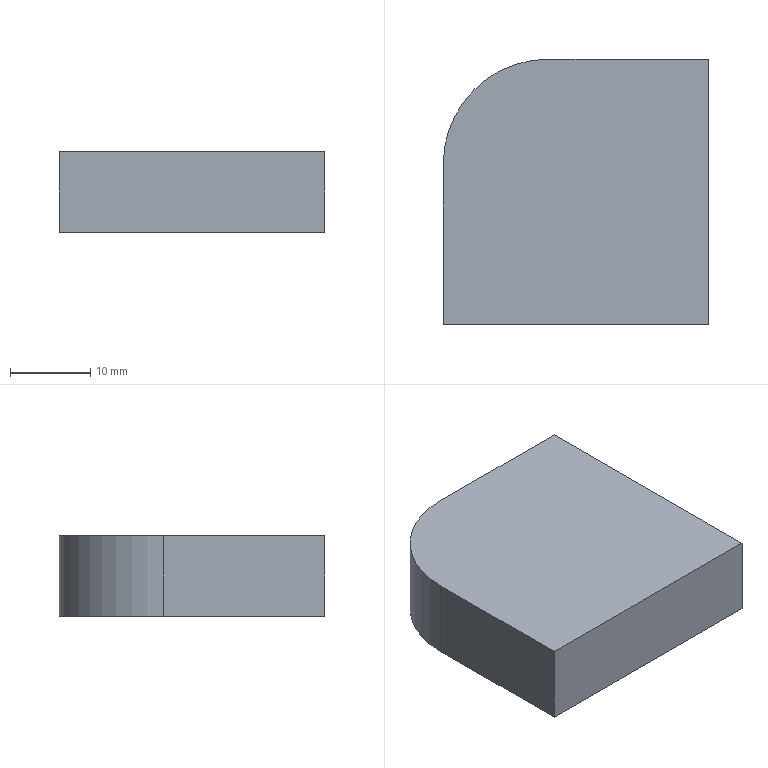Part | SolidWorks | features Extrusion 1, Fillet 1, ICE 1 | 1 solid | 7 faces | box 33 x 33 x 10 mm | volume 10527 mm3 | plane 6 | cylinder 1 | commonest cylinder face diameters 26 x1
STEP:
#1=CARTESIAN_POINT('',(7.,0.,10.));
#2=VERTEX_POINT('',#1);
#3=CARTESIAN_POINT('',(40.,0.,10.));
#4=VERTEX_POINT('',#3);
#5=CARTESIAN_POINT('',(40.,0.,10.));
#6=DIRECTION('',(1.,0.,0.));
#7=VECTOR('',#6,1000.);
#8=LINE('',#5,#7);
#9=EDGE_CURVE('',#2,#4,#8,.T.);
#10=ORIENTED_EDGE('',*,*,#9,.F.);
#11=CARTESIAN_POINT('',(7.,0.,0.));
#12=VERTEX_POINT('',#11);
#13=CARTESIAN_POINT('',(7.,0.,10.));
#14=DIRECTION('',(0.,0.,-1.));
#15=VECTOR('',#14,1000.);
#16=LINE('',#13,#15);
#17=EDGE_CURVE('',#2,#12,#16,.T.);
#18=ORIENTED_EDGE('',*,*,#17,.T.);
#19=CARTESIAN_POINT('',(40.,0.,0.));
#20=VERTEX_POINT('',#19);
#21=CARTESIAN_POINT('',(40.,0.,0.));
#22=DIRECTION('',(1.,0.,0.));
#23=VECTOR('',#22,1000.);
#24=LINE('',#21,#23);
#25=EDGE_CURVE('',#12,#20,#24,.T.);
#26=ORIENTED_EDGE('',*,*,#25,.T.);
#27=CARTESIAN_POINT('',(40.,0.,10.));
#28=DIRECTION('',(0.,0.,-1.));
#29=VECTOR('',#28,1000.);
#30=LINE('',#27,#29);
#31=EDGE_CURVE('',#4,#20,#30,.T.);
#32=ORIENTED_EDGE('',*,*,#31,.F.);
#33=EDGE_LOOP('',(#10,#18,#26,#32));
#34=FACE_OUTER_BOUND('',#33,.T.);
#35=CARTESIAN_POINT('',(40.,0.,10.));
#36=DIRECTION('',(0.,1.,0.));
#37=DIRECTION('',(0.,0.,1.));
#38=AXIS2_PLACEMENT_3D('',#35,#36,#37);
#39=PLANE('',#38);
#40=ADVANCED_FACE('',(#34),#39,.F.);
#41=CARTESIAN_POINT('',(40.,33.,0.));
#42=VERTEX_POINT('',#41);
#43=CARTESIAN_POINT('',(40.,40.,0.));
#44=DIRECTION('',(0.,1.,0.));
#45=VECTOR('',#44,1000.);
#46=LINE('',#43,#45);
#47=EDGE_CURVE('',#20,#42,#46,.T.);
#48=ORIENTED_EDGE('',*,*,#47,.T.);
#49=CARTESIAN_POINT('',(40.,33.,10.));
#50=VERTEX_POINT('',#49);
#51=CARTESIAN_POINT('',(40.,33.,10.));
#52=DIRECTION('',(0.,0.,-1.));
#53=VECTOR('',#52,1000.);
#54=LINE('',#51,#53);
#55=EDGE_CURVE('',#50,#42,#54,.T.);
#56=ORIENTED_EDGE('',*,*,#55,.F.);
#57=CARTESIAN_POINT('',(40.,40.,10.));
#58=DIRECTION('',(0.,1.,0.));
#59=VECTOR('',#58,1000.);
#60=LINE('',#57,#59);
#61=EDGE_CURVE('',#4,#50,#60,.T.);
#62=ORIENTED_EDGE('',*,*,#61,.F.);
#63=ORIENTED_EDGE('',*,*,#31,.T.);
#64=EDGE_LOOP('',(#48,#56,#62,#63));
#65=FACE_OUTER_BOUND('',#64,.T.);
#66=CARTESIAN_POINT('',(40.,40.,10.));
#67=DIRECTION('',(-1.,0.,0.));
#68=DIRECTION('',(0.,0.,1.));
#69=AXIS2_PLACEMENT_3D('',#66,#67,#68);
#70=PLANE('',#69);
#71=ADVANCED_FACE('',(#65),#70,.F.);
#72=CARTESIAN_POINT('',(20.,33.,10.));
#73=VERTEX_POINT('',#72);
#74=CARTESIAN_POINT('',(7.,20.,10.));
#75=VERTEX_POINT('',#74);
#76=CARTESIAN_POINT('',(20.,20.,10.));
#77=DIRECTION('',(0.,0.,1.));
#78=DIRECTION('',(-1.,0.,0.));
#79=AXIS2_PLACEMENT_3D('',#76,#77,#78);
#80=CIRCLE('',#79,13.);
#81=EDGE_CURVE('',#73,#75,#80,.T.);
#82=ORIENTED_EDGE('',*,*,#81,.T.);
#83=CARTESIAN_POINT('',(7.,20.,10.));
#84=DIRECTION('',(0.,-1.,0.));
#85=VECTOR('',#84,1000.);
#86=LINE('',#83,#85);
#87=EDGE_CURVE('',#75,#2,#86,.T.);
#88=ORIENTED_EDGE('',*,*,#87,.T.);
#89=ORIENTED_EDGE('',*,*,#9,.T.);
#90=ORIENTED_EDGE('',*,*,#61,.T.);
#91=CARTESIAN_POINT('',(40.,33.,10.));
#92=DIRECTION('',(-1.,0.,0.));
#93=VECTOR('',#92,1000.);
#94=LINE('',#91,#93);
#95=EDGE_CURVE('',#50,#73,#94,.T.);
#96=ORIENTED_EDGE('',*,*,#95,.T.);
#97=EDGE_LOOP('',(#82,#88,#89,#90,#96));
#98=FACE_OUTER_BOUND('',#97,.T.);
#99=CARTESIAN_POINT('',(0.,0.,10.));
#100=DIRECTION('',(0.,0.,-1.));
#101=DIRECTION('',(-1.,0.,0.));
#102=AXIS2_PLACEMENT_3D('',#99,#100,#101);
#103=PLANE('',#102);
#104=ADVANCED_FACE('',(#98),#103,.F.);
#105=CARTESIAN_POINT('',(7.,20.,0.));
#106=VERTEX_POINT('',#105);
#107=CARTESIAN_POINT('',(7.,20.,0.));
#108=DIRECTION('',(0.,-1.,0.));
#109=VECTOR('',#108,1000.);
#110=LINE('',#107,#109);
#111=EDGE_CURVE('',#106,#12,#110,.T.);
#112=ORIENTED_EDGE('',*,*,#111,.F.);
#113=CARTESIAN_POINT('',(20.,33.,0.));
#114=VERTEX_POINT('',#113);
#115=CARTESIAN_POINT('',(20.,20.,0.));
#116=DIRECTION('',(0.,0.,1.));
#117=DIRECTION('',(-1.,0.,0.));
#118=AXIS2_PLACEMENT_3D('',#115,#116,#117);
#119=CIRCLE('',#118,13.);
#120=EDGE_CURVE('',#114,#106,#119,.T.);
#121=ORIENTED_EDGE('',*,*,#120,.F.);
#122=CARTESIAN_POINT('',(40.,33.,0.));
#123=DIRECTION('',(-1.,0.,0.));
#124=VECTOR('',#123,1000.);
#125=LINE('',#122,#124);
#126=EDGE_CURVE('',#42,#114,#125,.T.);
#127=ORIENTED_EDGE('',*,*,#126,.F.);
#128=ORIENTED_EDGE('',*,*,#47,.F.);
#129=ORIENTED_EDGE('',*,*,#25,.F.);
#130=EDGE_LOOP('',(#112,#121,#127,#128,#129));
#131=FACE_OUTER_BOUND('',#130,.T.);
#132=CARTESIAN_POINT('',(0.,0.,0.));
#133=DIRECTION('',(0.,0.,-1.));
#134=DIRECTION('',(-1.,0.,0.));
#135=AXIS2_PLACEMENT_3D('',#132,#133,#134);
#136=PLANE('',#135);
#137=ADVANCED_FACE('',(#131),#136,.T.);
#138=ORIENTED_EDGE('',*,*,#111,.T.);
#139=ORIENTED_EDGE('',*,*,#17,.F.);
#140=ORIENTED_EDGE('',*,*,#87,.F.);
#141=CARTESIAN_POINT('',(7.,20.,10.));
#142=DIRECTION('',(0.,0.,-1.));
#143=VECTOR('',#142,1000.);
#144=LINE('',#141,#143);
#145=EDGE_CURVE('',#75,#106,#144,.T.);
#146=ORIENTED_EDGE('',*,*,#145,.T.);
#147=EDGE_LOOP('',(#138,#139,#140,#146));
#148=FACE_OUTER_BOUND('',#147,.T.);
#149=CARTESIAN_POINT('',(7.,20.,10.));
#150=DIRECTION('',(1.,0.,0.));
#151=DIRECTION('',(0.,1.,0.));
#152=AXIS2_PLACEMENT_3D('',#149,#150,#151);
#153=PLANE('',#152);
#154=ADVANCED_FACE('',(#148),#153,.F.);
#155=ORIENTED_EDGE('',*,*,#120,.T.);
#156=ORIENTED_EDGE('',*,*,#145,.F.);
#157=ORIENTED_EDGE('',*,*,#81,.F.);
#158=CARTESIAN_POINT('',(20.,33.,10.));
#159=DIRECTION('',(0.,0.,-1.));
#160=VECTOR('',#159,1000.);
#161=LINE('',#158,#160);
#162=EDGE_CURVE('',#73,#114,#161,.T.);
#163=ORIENTED_EDGE('',*,*,#162,.T.);
#164=EDGE_LOOP('',(#155,#156,#157,#163));
#165=FACE_OUTER_BOUND('',#164,.T.);
#166=CARTESIAN_POINT('',(20.,20.,10.));
#167=DIRECTION('',(0.,0.,-1.));
#168=DIRECTION('',(-1.,0.,0.));
#169=AXIS2_PLACEMENT_3D('',#166,#167,#168);
#170=CYLINDRICAL_SURFACE('',#169,13.);
#171=ADVANCED_FACE('',(#165),#170,.T.);
#172=ORIENTED_EDGE('',*,*,#126,.T.);
#173=ORIENTED_EDGE('',*,*,#162,.F.);
#174=ORIENTED_EDGE('',*,*,#95,.F.);
#175=ORIENTED_EDGE('',*,*,#55,.T.);
#176=EDGE_LOOP('',(#172,#173,#174,#175));
#177=FACE_OUTER_BOUND('',#176,.T.);
#178=CARTESIAN_POINT('',(40.,33.,10.));
#179=DIRECTION('',(0.,-1.,0.));
#180=DIRECTION('',(0.,0.,-1.));
#181=AXIS2_PLACEMENT_3D('',#178,#179,#180);
#182=PLANE('',#181);
#183=ADVANCED_FACE('',(#177),#182,.F.);
#184=CLOSED_SHELL('',(#40,#71,#104,#137,#154,#171,#183));
#185=MANIFOLD_SOLID_BREP('',#184);
#186=CARTESIAN_POINT('',(0.,0.,0.));
#187=DIRECTION('',(0.,0.,1.));
#188=DIRECTION('',(1.,0.,0.));
#189=AXIS2_PLACEMENT_3D('',#186,#187,#188);
#190=(LENGTH_UNIT()NAMED_UNIT(*)SI_UNIT(.MILLI.,.METRE.));
#191=UNCERTAINTY_MEASURE_WITH_UNIT(LENGTH_MEASURE(0.00001),#190,'','');
#192=(NAMED_UNIT(*)PLANE_ANGLE_UNIT()SI_UNIT($,.RADIAN.));
#193=(NAMED_UNIT(*)SI_UNIT($,.STERADIAN.)SOLID_ANGLE_UNIT());
#194=(GEOMETRIC_REPRESENTATION_CONTEXT(3)GLOBAL_UNCERTAINTY_ASSIGNED_CONTEXT((#191))GLOBAL_UNIT_ASSIGNED_CONTEXT((#190,#192,#193))REPRESENTATION_CONTEXT('',''));
#195=ADVANCED_BREP_SHAPE_REPRESENTATION('',(#185,#189),#194);